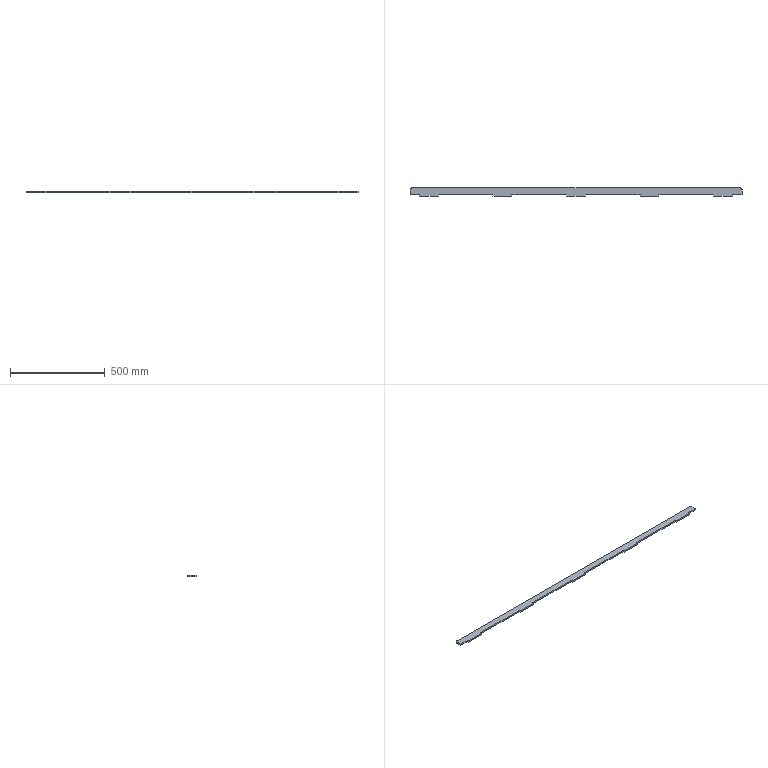Part | SolidWorks | features FlatPattern 1, SMBaseFlange 1, SheetMetal 1 | 1 solid | 28 faces | box 1750 x 42.5 x 8 mm | volume 519657 mm3 | plane 26 | cylinder 2 | commonest cylinder face diameters 20 x2
STEP:
#1=CARTESIAN_POINT('',(-889.737,-979.651,0.));
#2=VERTEX_POINT('',#1);
#3=CARTESIAN_POINT('',(-889.737,-1004.651,0.));
#4=VERTEX_POINT('',#3);
#5=CARTESIAN_POINT('',(-889.737,-1004.651,0.));
#6=DIRECTION('',(0.,-1.,0.));
#7=VECTOR('',#6,1000.);
#8=LINE('',#5,#7);
#9=EDGE_CURVE('',#2,#4,#8,.T.);
#10=ORIENTED_EDGE('',*,*,#9,.F.);
#11=CARTESIAN_POINT('',(-889.737,-979.651,-8.));
#12=VERTEX_POINT('',#11);
#13=CARTESIAN_POINT('',(-889.737,-979.651,-8.));
#14=DIRECTION('',(0.,0.,1.));
#15=VECTOR('',#14,1000.);
#16=LINE('',#13,#15);
#17=EDGE_CURVE('',#12,#2,#16,.T.);
#18=ORIENTED_EDGE('',*,*,#17,.F.);
#19=CARTESIAN_POINT('',(-889.737,-1004.651,-8.));
#20=VERTEX_POINT('',#19);
#21=CARTESIAN_POINT('',(-889.737,-1004.651,-8.));
#22=DIRECTION('',(0.,-1.,0.));
#23=VECTOR('',#22,1000.);
#24=LINE('',#21,#23);
#25=EDGE_CURVE('',#12,#20,#24,.T.);
#26=ORIENTED_EDGE('',*,*,#25,.T.);
#27=CARTESIAN_POINT('',(-889.737,-1004.651,-8.));
#28=DIRECTION('',(0.,0.,1.));
#29=VECTOR('',#28,1000.);
#30=LINE('',#27,#29);
#31=EDGE_CURVE('',#20,#4,#30,.T.);
#32=ORIENTED_EDGE('',*,*,#31,.T.);
#33=EDGE_LOOP('',(#10,#18,#26,#32));
#34=FACE_OUTER_BOUND('',#33,.T.);
#35=CARTESIAN_POINT('',(-889.737,-1004.651,-8.));
#36=DIRECTION('',(-1.,0.,0.));
#37=DIRECTION('',(0.,0.,1.));
#38=AXIS2_PLACEMENT_3D('',#35,#36,#37);
#39=PLANE('',#38);
#40=ADVANCED_FACE('',(#34),#39,.T.);
#41=CARTESIAN_POINT('',(-879.737,-969.651,0.));
#42=VERTEX_POINT('',#41);
#43=CARTESIAN_POINT('',(-879.737,-979.651,0.));
#44=DIRECTION('',(0.,0.,1.));
#45=DIRECTION('',(-1.,0.,0.));
#46=AXIS2_PLACEMENT_3D('',#43,#44,#45);
#47=CIRCLE('',#46,10.);
#48=EDGE_CURVE('',#42,#2,#47,.T.);
#49=ORIENTED_EDGE('',*,*,#48,.F.);
#50=CARTESIAN_POINT('',(-879.737,-969.651,-8.));
#51=VERTEX_POINT('',#50);
#52=CARTESIAN_POINT('',(-879.737,-969.651,-8.));
#53=DIRECTION('',(0.,0.,1.));
#54=VECTOR('',#53,1000.);
#55=LINE('',#52,#54);
#56=EDGE_CURVE('',#51,#42,#55,.T.);
#57=ORIENTED_EDGE('',*,*,#56,.F.);
#58=CARTESIAN_POINT('',(-879.737,-979.651,-8.));
#59=DIRECTION('',(0.,0.,1.));
#60=DIRECTION('',(-1.,0.,0.));
#61=AXIS2_PLACEMENT_3D('',#58,#59,#60);
#62=CIRCLE('',#61,10.);
#63=EDGE_CURVE('',#51,#12,#62,.T.);
#64=ORIENTED_EDGE('',*,*,#63,.T.);
#65=ORIENTED_EDGE('',*,*,#17,.T.);
#66=EDGE_LOOP('',(#49,#57,#64,#65));
#67=FACE_OUTER_BOUND('',#66,.T.);
#68=CARTESIAN_POINT('',(-879.737,-979.651,-8.));
#69=DIRECTION('',(0.,0.,1.));
#70=DIRECTION('',(1.,0.,0.));
#71=AXIS2_PLACEMENT_3D('',#68,#69,#70);
#72=CYLINDRICAL_SURFACE('',#71,10.);
#73=ADVANCED_FACE('',(#67),#72,.T.);
#74=CARTESIAN_POINT('',(850.263,-969.651,0.));
#75=VERTEX_POINT('',#74);
#76=CARTESIAN_POINT('',(-879.737,-969.651,0.));
#77=DIRECTION('',(-1.,0.,0.));
#78=VECTOR('',#77,1000.);
#79=LINE('',#76,#78);
#80=EDGE_CURVE('',#75,#42,#79,.T.);
#81=ORIENTED_EDGE('',*,*,#80,.F.);
#82=CARTESIAN_POINT('',(850.263,-969.651,-8.));
#83=VERTEX_POINT('',#82);
#84=CARTESIAN_POINT('',(850.263,-969.651,-8.));
#85=DIRECTION('',(0.,0.,1.));
#86=VECTOR('',#85,1000.);
#87=LINE('',#84,#86);
#88=EDGE_CURVE('',#83,#75,#87,.T.);
#89=ORIENTED_EDGE('',*,*,#88,.F.);
#90=CARTESIAN_POINT('',(-879.737,-969.651,-8.));
#91=DIRECTION('',(-1.,0.,0.));
#92=VECTOR('',#91,1000.);
#93=LINE('',#90,#92);
#94=EDGE_CURVE('',#83,#51,#93,.T.);
#95=ORIENTED_EDGE('',*,*,#94,.T.);
#96=ORIENTED_EDGE('',*,*,#56,.T.);
#97=EDGE_LOOP('',(#81,#89,#95,#96));
#98=FACE_OUTER_BOUND('',#97,.T.);
#99=CARTESIAN_POINT('',(-879.737,-969.651,-8.));
#100=DIRECTION('',(0.,1.,0.));
#101=DIRECTION('',(0.,0.,1.));
#102=AXIS2_PLACEMENT_3D('',#99,#100,#101);
#103=PLANE('',#102);
#104=ADVANCED_FACE('',(#98),#103,.T.);
#105=CARTESIAN_POINT('',(860.263,-979.651,0.));
#106=VERTEX_POINT('',#105);
#107=CARTESIAN_POINT('',(850.263,-979.651,0.));
#108=DIRECTION('',(0.,0.,1.));
#109=DIRECTION('',(-1.,0.,0.));
#110=AXIS2_PLACEMENT_3D('',#107,#108,#109);
#111=CIRCLE('',#110,10.);
#112=EDGE_CURVE('',#106,#75,#111,.T.);
#113=ORIENTED_EDGE('',*,*,#112,.F.);
#114=CARTESIAN_POINT('',(860.263,-979.651,-8.));
#115=VERTEX_POINT('',#114);
#116=CARTESIAN_POINT('',(860.263,-979.651,-8.));
#117=DIRECTION('',(0.,0.,1.));
#118=VECTOR('',#117,1000.);
#119=LINE('',#116,#118);
#120=EDGE_CURVE('',#115,#106,#119,.T.);
#121=ORIENTED_EDGE('',*,*,#120,.F.);
#122=CARTESIAN_POINT('',(850.263,-979.651,-8.));
#123=DIRECTION('',(0.,0.,1.));
#124=DIRECTION('',(-1.,0.,0.));
#125=AXIS2_PLACEMENT_3D('',#122,#123,#124);
#126=CIRCLE('',#125,10.);
#127=EDGE_CURVE('',#115,#83,#126,.T.);
#128=ORIENTED_EDGE('',*,*,#127,.T.);
#129=ORIENTED_EDGE('',*,*,#88,.T.);
#130=EDGE_LOOP('',(#113,#121,#128,#129));
#131=FACE_OUTER_BOUND('',#130,.T.);
#132=CARTESIAN_POINT('',(850.263,-979.651,-8.));
#133=DIRECTION('',(0.,0.,1.));
#134=DIRECTION('',(1.,0.,0.));
#135=AXIS2_PLACEMENT_3D('',#132,#133,#134);
#136=CYLINDRICAL_SURFACE('',#135,10.);
#137=ADVANCED_FACE('',(#131),#136,.T.);
#138=CARTESIAN_POINT('',(860.263,-1004.651,0.));
#139=VERTEX_POINT('',#138);
#140=CARTESIAN_POINT('',(860.263,-1004.651,0.));
#141=DIRECTION('',(0.,1.,0.));
#142=VECTOR('',#141,1000.);
#143=LINE('',#140,#142);
#144=EDGE_CURVE('',#139,#106,#143,.T.);
#145=ORIENTED_EDGE('',*,*,#144,.F.);
#146=CARTESIAN_POINT('',(860.263,-1004.651,-8.));
#147=VERTEX_POINT('',#146);
#148=CARTESIAN_POINT('',(860.263,-1004.651,-8.));
#149=DIRECTION('',(0.,0.,1.));
#150=VECTOR('',#149,1000.);
#151=LINE('',#148,#150);
#152=EDGE_CURVE('',#147,#139,#151,.T.);
#153=ORIENTED_EDGE('',*,*,#152,.F.);
#154=CARTESIAN_POINT('',(860.263,-1004.651,-8.));
#155=DIRECTION('',(0.,1.,0.));
#156=VECTOR('',#155,1000.);
#157=LINE('',#154,#156);
#158=EDGE_CURVE('',#147,#115,#157,.T.);
#159=ORIENTED_EDGE('',*,*,#158,.T.);
#160=ORIENTED_EDGE('',*,*,#120,.T.);
#161=EDGE_LOOP('',(#145,#153,#159,#160));
#162=FACE_OUTER_BOUND('',#161,.T.);
#163=CARTESIAN_POINT('',(860.263,-1004.651,-8.));
#164=DIRECTION('',(1.,0.,0.));
#165=DIRECTION('',(0.,0.,-1.));
#166=AXIS2_PLACEMENT_3D('',#163,#164,#165);
#167=PLANE('',#166);
#168=ADVANCED_FACE('',(#162),#167,.T.);
#169=CARTESIAN_POINT('',(810.263,-1004.651,0.));
#170=VERTEX_POINT('',#169);
#171=CARTESIAN_POINT('',(810.263,-1004.651,0.));
#172=DIRECTION('',(1.,0.,0.));
#173=VECTOR('',#172,1000.);
#174=LINE('',#171,#173);
#175=EDGE_CURVE('',#170,#139,#174,.T.);
#176=ORIENTED_EDGE('',*,*,#175,.F.);
#177=CARTESIAN_POINT('',(810.263,-1004.651,-8.));
#178=VERTEX_POINT('',#177);
#179=CARTESIAN_POINT('',(810.263,-1004.651,-8.));
#180=DIRECTION('',(0.,0.,1.));
#181=VECTOR('',#180,1000.);
#182=LINE('',#179,#181);
#183=EDGE_CURVE('',#178,#170,#182,.T.);
#184=ORIENTED_EDGE('',*,*,#183,.F.);
#185=CARTESIAN_POINT('',(810.263,-1004.651,-8.));
#186=DIRECTION('',(1.,0.,0.));
#187=VECTOR('',#186,1000.);
#188=LINE('',#185,#187);
#189=EDGE_CURVE('',#178,#147,#188,.T.);
#190=ORIENTED_EDGE('',*,*,#189,.T.);
#191=ORIENTED_EDGE('',*,*,#152,.T.);
#192=EDGE_LOOP('',(#176,#184,#190,#191));
#193=FACE_OUTER_BOUND('',#192,.T.);
#194=CARTESIAN_POINT('',(810.263,-1004.651,-8.));
#195=DIRECTION('',(0.,-1.,0.));
#196=DIRECTION('',(0.,0.,-1.));
#197=AXIS2_PLACEMENT_3D('',#194,#195,#196);
#198=PLANE('',#197);
#199=ADVANCED_FACE('',(#193),#198,.T.);
#200=CARTESIAN_POINT('',(810.263,-1012.151,0.));
#201=VERTEX_POINT('',#200);
#202=CARTESIAN_POINT('',(810.263,-1004.651,0.));
#203=DIRECTION('',(0.,1.,0.));
#204=VECTOR('',#203,1000.);
#205=LINE('',#202,#204);
#206=EDGE_CURVE('',#201,#170,#205,.T.);
#207=ORIENTED_EDGE('',*,*,#206,.F.);
#208=CARTESIAN_POINT('',(810.263,-1012.151,-8.));
#209=VERTEX_POINT('',#208);
#210=CARTESIAN_POINT('',(810.263,-1012.151,-8.));
#211=DIRECTION('',(0.,0.,1.));
#212=VECTOR('',#211,1000.);
#213=LINE('',#210,#212);
#214=EDGE_CURVE('',#209,#201,#213,.T.);
#215=ORIENTED_EDGE('',*,*,#214,.F.);
#216=CARTESIAN_POINT('',(810.263,-1004.651,-8.));
#217=DIRECTION('',(0.,1.,0.));
#218=VECTOR('',#217,1000.);
#219=LINE('',#216,#218);
#220=EDGE_CURVE('',#209,#178,#219,.T.);
#221=ORIENTED_EDGE('',*,*,#220,.T.);
#222=ORIENTED_EDGE('',*,*,#183,.T.);
#223=EDGE_LOOP('',(#207,#215,#221,#222));
#224=FACE_OUTER_BOUND('',#223,.T.);
#225=CARTESIAN_POINT('',(810.263,-1004.651,-8.));
#226=DIRECTION('',(1.,0.,0.));
#227=DIRECTION('',(0.,0.,-1.));
#228=AXIS2_PLACEMENT_3D('',#225,#226,#227);
#229=PLANE('',#228);
#230=ADVANCED_FACE('',(#224),#229,.T.);
#231=CARTESIAN_POINT('',(710.263,-1012.151,0.));
#232=VERTEX_POINT('',#231);
#233=CARTESIAN_POINT('',(810.263,-1012.151,0.));
#234=DIRECTION('',(1.,0.,0.));
#235=VECTOR('',#234,1000.);
#236=LINE('',#233,#235);
#237=EDGE_CURVE('',#232,#201,#236,.T.);
#238=ORIENTED_EDGE('',*,*,#237,.F.);
#239=CARTESIAN_POINT('',(710.263,-1012.151,-8.));
#240=VERTEX_POINT('',#239);
#241=CARTESIAN_POINT('',(710.263,-1012.151,-8.));
#242=DIRECTION('',(0.,0.,1.));
#243=VECTOR('',#242,1000.);
#244=LINE('',#241,#243);
#245=EDGE_CURVE('',#240,#232,#244,.T.);
#246=ORIENTED_EDGE('',*,*,#245,.F.);
#247=CARTESIAN_POINT('',(810.263,-1012.151,-8.));
#248=DIRECTION('',(1.,0.,0.));
#249=VECTOR('',#248,1000.);
#250=LINE('',#247,#249);
#251=EDGE_CURVE('',#240,#209,#250,.T.);
#252=ORIENTED_EDGE('',*,*,#251,.T.);
#253=ORIENTED_EDGE('',*,*,#214,.T.);
#254=EDGE_LOOP('',(#238,#246,#252,#253));
#255=FACE_OUTER_BOUND('',#254,.T.);
#256=CARTESIAN_POINT('',(810.263,-1012.151,-8.));
#257=DIRECTION('',(0.,-1.,0.));
#258=DIRECTION('',(0.,0.,-1.));
#259=AXIS2_PLACEMENT_3D('',#256,#257,#258);
#260=PLANE('',#259);
#261=ADVANCED_FACE('',(#255),#260,.T.);
#262=CARTESIAN_POINT('',(710.263,-1004.651,0.));
#263=VERTEX_POINT('',#262);
#264=CARTESIAN_POINT('',(710.263,-1012.151,0.));
#265=DIRECTION('',(0.,-1.,0.));
#266=VECTOR('',#265,1000.);
#267=LINE('',#264,#266);
#268=EDGE_CURVE('',#263,#232,#267,.T.);
#269=ORIENTED_EDGE('',*,*,#268,.F.);
#270=CARTESIAN_POINT('',(710.263,-1004.651,-8.));
#271=VERTEX_POINT('',#270);
#272=CARTESIAN_POINT('',(710.263,-1004.651,-8.));
#273=DIRECTION('',(0.,0.,1.));
#274=VECTOR('',#273,1000.);
#275=LINE('',#272,#274);
#276=EDGE_CURVE('',#271,#263,#275,.T.);
#277=ORIENTED_EDGE('',*,*,#276,.F.);
#278=CARTESIAN_POINT('',(710.263,-1012.151,-8.));
#279=DIRECTION('',(0.,-1.,0.));
#280=VECTOR('',#279,1000.);
#281=LINE('',#278,#280);
#282=EDGE_CURVE('',#271,#240,#281,.T.);
#283=ORIENTED_EDGE('',*,*,#282,.T.);
#284=ORIENTED_EDGE('',*,*,#245,.T.);
#285=EDGE_LOOP('',(#269,#277,#283,#284));
#286=FACE_OUTER_BOUND('',#285,.T.);
#287=CARTESIAN_POINT('',(710.263,-1012.151,-8.));
#288=DIRECTION('',(-1.,0.,0.));
#289=DIRECTION('',(0.,0.,1.));
#290=AXIS2_PLACEMENT_3D('',#287,#288,#289);
#291=PLANE('',#290);
#292=ADVANCED_FACE('',(#286),#291,.T.);
#293=CARTESIAN_POINT('',(422.763,-1004.651,0.));
#294=VERTEX_POINT('',#293);
#295=CARTESIAN_POINT('',(422.763,-1004.651,0.));
#296=DIRECTION('',(1.,0.,0.));
#297=VECTOR('',#296,1000.);
#298=LINE('',#295,#297);
#299=EDGE_CURVE('',#294,#263,#298,.T.);
#300=ORIENTED_EDGE('',*,*,#299,.F.);
#301=CARTESIAN_POINT('',(422.763,-1004.651,-8.));
#302=VERTEX_POINT('',#301);
#303=CARTESIAN_POINT('',(422.763,-1004.651,-8.));
#304=DIRECTION('',(0.,0.,1.));
#305=VECTOR('',#304,1000.);
#306=LINE('',#303,#305);
#307=EDGE_CURVE('',#302,#294,#306,.T.);
#308=ORIENTED_EDGE('',*,*,#307,.F.);
#309=CARTESIAN_POINT('',(422.763,-1004.651,-8.));
#310=DIRECTION('',(1.,0.,0.));
#311=VECTOR('',#310,1000.);
#312=LINE('',#309,#311);
#313=EDGE_CURVE('',#302,#271,#312,.T.);
#314=ORIENTED_EDGE('',*,*,#313,.T.);
#315=ORIENTED_EDGE('',*,*,#276,.T.);
#316=EDGE_LOOP('',(#300,#308,#314,#315));
#317=FACE_OUTER_BOUND('',#316,.T.);
#318=CARTESIAN_POINT('',(422.763,-1004.651,-8.));
#319=DIRECTION('',(0.,-1.,0.));
#320=DIRECTION('',(0.,0.,-1.));
#321=AXIS2_PLACEMENT_3D('',#318,#319,#320);
#322=PLANE('',#321);
#323=ADVANCED_FACE('',(#317),#322,.T.);
#324=CARTESIAN_POINT('',(422.763,-1012.151,0.));
#325=VERTEX_POINT('',#324);
#326=CARTESIAN_POINT('',(422.763,-1012.151,0.));
#327=DIRECTION('',(0.,1.,0.));
#328=VECTOR('',#327,1000.);
#329=LINE('',#326,#328);
#330=EDGE_CURVE('',#325,#294,#329,.T.);
#331=ORIENTED_EDGE('',*,*,#330,.F.);
#332=CARTESIAN_POINT('',(422.763,-1012.151,-8.));
#333=VERTEX_POINT('',#332);
#334=CARTESIAN_POINT('',(422.763,-1012.151,-8.));
#335=DIRECTION('',(0.,0.,1.));
#336=VECTOR('',#335,1000.);
#337=LINE('',#334,#336);
#338=EDGE_CURVE('',#333,#325,#337,.T.);
#339=ORIENTED_EDGE('',*,*,#338,.F.);
#340=CARTESIAN_POINT('',(422.763,-1012.151,-8.));
#341=DIRECTION('',(0.,1.,0.));
#342=VECTOR('',#341,1000.);
#343=LINE('',#340,#342);
#344=EDGE_CURVE('',#333,#302,#343,.T.);
#345=ORIENTED_EDGE('',*,*,#344,.T.);
#346=ORIENTED_EDGE('',*,*,#307,.T.);
#347=EDGE_LOOP('',(#331,#339,#345,#346));
#348=FACE_OUTER_BOUND('',#347,.T.);
#349=CARTESIAN_POINT('',(422.763,-1012.151,-8.));
#350=DIRECTION('',(1.,0.,0.));
#351=DIRECTION('',(0.,0.,-1.));
#352=AXIS2_PLACEMENT_3D('',#349,#350,#351);
#353=PLANE('',#352);
#354=ADVANCED_FACE('',(#348),#353,.T.);
#355=CARTESIAN_POINT('',(322.763,-1012.151,0.));
#356=VERTEX_POINT('',#355);
#357=CARTESIAN_POINT('',(322.763,-1012.151,0.));
#358=DIRECTION('',(1.,0.,0.));
#359=VECTOR('',#358,1000.);
#360=LINE('',#357,#359);
#361=EDGE_CURVE('',#356,#325,#360,.T.);
#362=ORIENTED_EDGE('',*,*,#361,.F.);
#363=CARTESIAN_POINT('',(322.763,-1012.151,-8.));
#364=VERTEX_POINT('',#363);
#365=CARTESIAN_POINT('',(322.763,-1012.151,-8.));
#366=DIRECTION('',(0.,0.,1.));
#367=VECTOR('',#366,1000.);
#368=LINE('',#365,#367);
#369=EDGE_CURVE('',#364,#356,#368,.T.);
#370=ORIENTED_EDGE('',*,*,#369,.F.);
#371=CARTESIAN_POINT('',(322.763,-1012.151,-8.));
#372=DIRECTION('',(1.,0.,0.));
#373=VECTOR('',#372,1000.);
#374=LINE('',#371,#373);
#375=EDGE_CURVE('',#364,#333,#374,.T.);
#376=ORIENTED_EDGE('',*,*,#375,.T.);
#377=ORIENTED_EDGE('',*,*,#338,.T.);
#378=EDGE_LOOP('',(#362,#370,#376,#377));
#379=FACE_OUTER_BOUND('',#378,.T.);
#380=CARTESIAN_POINT('',(322.763,-1012.151,-8.));
#381=DIRECTION('',(0.,-1.,0.));
#382=DIRECTION('',(0.,0.,-1.));
#383=AXIS2_PLACEMENT_3D('',#380,#381,#382);
#384=PLANE('',#383);
#385=ADVANCED_FACE('',(#379),#384,.T.);
#386=CARTESIAN_POINT('',(322.763,-1004.651,0.));
#387=VERTEX_POINT('',#386);
#388=CARTESIAN_POINT('',(322.763,-1004.651,0.));
#389=DIRECTION('',(0.,-1.,0.));
#390=VECTOR('',#389,1000.);
#391=LINE('',#388,#390);
#392=EDGE_CURVE('',#387,#356,#391,.T.);
#393=ORIENTED_EDGE('',*,*,#392,.F.);
#394=CARTESIAN_POINT('',(322.763,-1004.651,-8.));
#395=VERTEX_POINT('',#394);
#396=CARTESIAN_POINT('',(322.763,-1004.651,-8.));
#397=DIRECTION('',(0.,0.,1.));
#398=VECTOR('',#397,1000.);
#399=LINE('',#396,#398);
#400=EDGE_CURVE('',#395,#387,#399,.T.);
#401=ORIENTED_EDGE('',*,*,#400,.F.);
#402=CARTESIAN_POINT('',(322.763,-1004.651,-8.));
#403=DIRECTION('',(0.,-1.,0.));
#404=VECTOR('',#403,1000.);
#405=LINE('',#402,#404);
#406=EDGE_CURVE('',#395,#364,#405,.T.);
#407=ORIENTED_EDGE('',*,*,#406,.T.);
#408=ORIENTED_EDGE('',*,*,#369,.T.);
#409=EDGE_LOOP('',(#393,#401,#407,#408));
#410=FACE_OUTER_BOUND('',#409,.T.);
#411=CARTESIAN_POINT('',(322.763,-1004.651,-8.));
#412=DIRECTION('',(-1.,0.,0.));
#413=DIRECTION('',(0.,0.,1.));
#414=AXIS2_PLACEMENT_3D('',#411,#412,#413);
#415=PLANE('',#414);
#416=ADVANCED_FACE('',(#410),#415,.T.);
#417=CARTESIAN_POINT('',(35.263,-1004.651,0.));
#418=VERTEX_POINT('',#417);
#419=CARTESIAN_POINT('',(35.263,-1004.651,0.));
#420=DIRECTION('',(1.,0.,0.));
#421=VECTOR('',#420,1000.);
#422=LINE('',#419,#421);
#423=EDGE_CURVE('',#418,#387,#422,.T.);
#424=ORIENTED_EDGE('',*,*,#423,.F.);
#425=CARTESIAN_POINT('',(35.263,-1004.651,-8.));
#426=VERTEX_POINT('',#425);
#427=CARTESIAN_POINT('',(35.263,-1004.651,-8.));
#428=DIRECTION('',(0.,0.,1.));
#429=VECTOR('',#428,1000.);
#430=LINE('',#427,#429);
#431=EDGE_CURVE('',#426,#418,#430,.T.);
#432=ORIENTED_EDGE('',*,*,#431,.F.);
#433=CARTESIAN_POINT('',(35.263,-1004.651,-8.));
#434=DIRECTION('',(1.,0.,0.));
#435=VECTOR('',#434,1000.);
#436=LINE('',#433,#435);
#437=EDGE_CURVE('',#426,#395,#436,.T.);
#438=ORIENTED_EDGE('',*,*,#437,.T.);
#439=ORIENTED_EDGE('',*,*,#400,.T.);
#440=EDGE_LOOP('',(#424,#432,#438,#439));
#441=FACE_OUTER_BOUND('',#440,.T.);
#442=CARTESIAN_POINT('',(35.263,-1004.651,-8.));
#443=DIRECTION('',(0.,-1.,0.));
#444=DIRECTION('',(0.,0.,-1.));
#445=AXIS2_PLACEMENT_3D('',#442,#443,#444);
#446=PLANE('',#445);
#447=ADVANCED_FACE('',(#441),#446,.T.);
#448=CARTESIAN_POINT('',(35.263,-1012.151,0.));
#449=VERTEX_POINT('',#448);
#450=CARTESIAN_POINT('',(35.263,-1012.151,0.));
#451=DIRECTION('',(0.,1.,0.));
#452=VECTOR('',#451,1000.);
#453=LINE('',#450,#452);
#454=EDGE_CURVE('',#449,#418,#453,.T.);
#455=ORIENTED_EDGE('',*,*,#454,.F.);
#456=CARTESIAN_POINT('',(35.263,-1012.151,-8.));
#457=VERTEX_POINT('',#456);
#458=CARTESIAN_POINT('',(35.263,-1012.151,-8.));
#459=DIRECTION('',(0.,0.,1.));
#460=VECTOR('',#459,1000.);
#461=LINE('',#458,#460);
#462=EDGE_CURVE('',#457,#449,#461,.T.);
#463=ORIENTED_EDGE('',*,*,#462,.F.);
#464=CARTESIAN_POINT('',(35.263,-1012.151,-8.));
#465=DIRECTION('',(0.,1.,0.));
#466=VECTOR('',#465,1000.);
#467=LINE('',#464,#466);
#468=EDGE_CURVE('',#457,#426,#467,.T.);
#469=ORIENTED_EDGE('',*,*,#468,.T.);
#470=ORIENTED_EDGE('',*,*,#431,.T.);
#471=EDGE_LOOP('',(#455,#463,#469,#470));
#472=FACE_OUTER_BOUND('',#471,.T.);
#473=CARTESIAN_POINT('',(35.263,-1012.151,-8.));
#474=DIRECTION('',(1.,0.,0.));
#475=DIRECTION('',(0.,0.,-1.));
#476=AXIS2_PLACEMENT_3D('',#473,#474,#475);
#477=PLANE('',#476);
#478=ADVANCED_FACE('',(#472),#477,.T.);
#479=CARTESIAN_POINT('',(-64.737,-1012.151,0.));
#480=VERTEX_POINT('',#479);
#481=CARTESIAN_POINT('',(-64.737,-1012.151,0.));
#482=DIRECTION('',(1.,0.,0.));
#483=VECTOR('',#482,1000.);
#484=LINE('',#481,#483);
#485=EDGE_CURVE('',#480,#449,#484,.T.);
#486=ORIENTED_EDGE('',*,*,#485,.F.);
#487=CARTESIAN_POINT('',(-64.737,-1012.151,-8.));
#488=VERTEX_POINT('',#487);
#489=CARTESIAN_POINT('',(-64.737,-1012.151,-8.));
#490=DIRECTION('',(0.,0.,1.));
#491=VECTOR('',#490,1000.);
#492=LINE('',#489,#491);
#493=EDGE_CURVE('',#488,#480,#492,.T.);
#494=ORIENTED_EDGE('',*,*,#493,.F.);
#495=CARTESIAN_POINT('',(-64.737,-1012.151,-8.));
#496=DIRECTION('',(1.,0.,0.));
#497=VECTOR('',#496,1000.);
#498=LINE('',#495,#497);
#499=EDGE_CURVE('',#488,#457,#498,.T.);
#500=ORIENTED_EDGE('',*,*,#499,.T.);
#501=ORIENTED_EDGE('',*,*,#462,.T.);
#502=EDGE_LOOP('',(#486,#494,#500,#501));
#503=FACE_OUTER_BOUND('',#502,.T.);
#504=CARTESIAN_POINT('',(-64.737,-1012.151,-8.));
#505=DIRECTION('',(0.,-1.,0.));
#506=DIRECTION('',(0.,0.,-1.));
#507=AXIS2_PLACEMENT_3D('',#504,#505,#506);
#508=PLANE('',#507);
#509=ADVANCED_FACE('',(#503),#508,.T.);
#510=CARTESIAN_POINT('',(-64.737,-1004.651,0.));
#511=VERTEX_POINT('',#510);
#512=CARTESIAN_POINT('',(-64.737,-1004.651,0.));
#513=DIRECTION('',(0.,-1.,0.));
#514=VECTOR('',#513,1000.);
#515=LINE('',#512,#514);
#516=EDGE_CURVE('',#511,#480,#515,.T.);
#517=ORIENTED_EDGE('',*,*,#516,.F.);
#518=CARTESIAN_POINT('',(-64.737,-1004.651,-8.));
#519=VERTEX_POINT('',#518);
#520=CARTESIAN_POINT('',(-64.737,-1004.651,-8.));
#521=DIRECTION('',(0.,0.,1.));
#522=VECTOR('',#521,1000.);
#523=LINE('',#520,#522);
#524=EDGE_CURVE('',#519,#511,#523,.T.);
#525=ORIENTED_EDGE('',*,*,#524,.F.);
#526=CARTESIAN_POINT('',(-64.737,-1004.651,-8.));
#527=DIRECTION('',(0.,-1.,0.));
#528=VECTOR('',#527,1000.);
#529=LINE('',#526,#528);
#530=EDGE_CURVE('',#519,#488,#529,.T.);
#531=ORIENTED_EDGE('',*,*,#530,.T.);
#532=ORIENTED_EDGE('',*,*,#493,.T.);
#533=EDGE_LOOP('',(#517,#525,#531,#532));
#534=FACE_OUTER_BOUND('',#533,.T.);
#535=CARTESIAN_POINT('',(-64.737,-1004.651,-8.));
#536=DIRECTION('',(-1.,0.,0.));
#537=DIRECTION('',(0.,-1.,0.));
#538=AXIS2_PLACEMENT_3D('',#535,#536,#537);
#539=PLANE('',#538);
#540=ADVANCED_FACE('',(#534),#539,.T.);
#541=CARTESIAN_POINT('',(-352.237,-1004.651,0.));
#542=VERTEX_POINT('',#541);
#543=CARTESIAN_POINT('',(-352.237,-1004.651,0.));
#544=DIRECTION('',(1.,0.,0.));
#545=VECTOR('',#544,1000.);
#546=LINE('',#543,#545);
#547=EDGE_CURVE('',#542,#511,#546,.T.);
#548=ORIENTED_EDGE('',*,*,#547,.F.);
#549=CARTESIAN_POINT('',(-352.237,-1004.651,-8.));
#550=VERTEX_POINT('',#549);
#551=CARTESIAN_POINT('',(-352.237,-1004.651,-8.));
#552=DIRECTION('',(0.,0.,1.));
#553=VECTOR('',#552,1000.);
#554=LINE('',#551,#553);
#555=EDGE_CURVE('',#550,#542,#554,.T.);
#556=ORIENTED_EDGE('',*,*,#555,.F.);
#557=CARTESIAN_POINT('',(-352.237,-1004.651,-8.));
#558=DIRECTION('',(1.,0.,0.));
#559=VECTOR('',#558,1000.);
#560=LINE('',#557,#559);
#561=EDGE_CURVE('',#550,#519,#560,.T.);
#562=ORIENTED_EDGE('',*,*,#561,.T.);
#563=ORIENTED_EDGE('',*,*,#524,.T.);
#564=EDGE_LOOP('',(#548,#556,#562,#563));
#565=FACE_OUTER_BOUND('',#564,.T.);
#566=CARTESIAN_POINT('',(-352.237,-1004.651,-8.));
#567=DIRECTION('',(0.,-1.,0.));
#568=DIRECTION('',(0.,0.,-1.));
#569=AXIS2_PLACEMENT_3D('',#566,#567,#568);
#570=PLANE('',#569);
#571=ADVANCED_FACE('',(#565),#570,.T.);
#572=CARTESIAN_POINT('',(-352.237,-1012.151,0.));
#573=VERTEX_POINT('',#572);
#574=CARTESIAN_POINT('',(-352.237,-1012.151,0.));
#575=DIRECTION('',(0.,1.,0.));
#576=VECTOR('',#575,1000.);
#577=LINE('',#574,#576);
#578=EDGE_CURVE('',#573,#542,#577,.T.);
#579=ORIENTED_EDGE('',*,*,#578,.F.);
#580=CARTESIAN_POINT('',(-352.237,-1012.151,-8.));
#581=VERTEX_POINT('',#580);
#582=CARTESIAN_POINT('',(-352.237,-1012.151,-8.));
#583=DIRECTION('',(0.,0.,1.));
#584=VECTOR('',#583,1000.);
#585=LINE('',#582,#584);
#586=EDGE_CURVE('',#581,#573,#585,.T.);
#587=ORIENTED_EDGE('',*,*,#586,.F.);
#588=CARTESIAN_POINT('',(-352.237,-1012.151,-8.));
#589=DIRECTION('',(0.,1.,0.));
#590=VECTOR('',#589,1000.);
#591=LINE('',#588,#590);
#592=EDGE_CURVE('',#581,#550,#591,.T.);
#593=ORIENTED_EDGE('',*,*,#592,.T.);
#594=ORIENTED_EDGE('',*,*,#555,.T.);
#595=EDGE_LOOP('',(#579,#587,#593,#594));
#596=FACE_OUTER_BOUND('',#595,.T.);
#597=CARTESIAN_POINT('',(-352.237,-1012.151,-8.));
#598=DIRECTION('',(1.,0.,0.));
#599=DIRECTION('',(0.,0.,-1.));
#600=AXIS2_PLACEMENT_3D('',#597,#598,#599);
#601=PLANE('',#600);
#602=ADVANCED_FACE('',(#596),#601,.T.);
#603=CARTESIAN_POINT('',(-452.237,-1012.151,0.));
#604=VERTEX_POINT('',#603);
#605=CARTESIAN_POINT('',(-452.237,-1012.151,0.));
#606=DIRECTION('',(1.,0.,0.));
#607=VECTOR('',#606,1000.);
#608=LINE('',#605,#607);
#609=EDGE_CURVE('',#604,#573,#608,.T.);
#610=ORIENTED_EDGE('',*,*,#609,.F.);
#611=CARTESIAN_POINT('',(-452.237,-1012.151,-8.));
#612=VERTEX_POINT('',#611);
#613=CARTESIAN_POINT('',(-452.237,-1012.151,-8.));
#614=DIRECTION('',(0.,0.,1.));
#615=VECTOR('',#614,1000.);
#616=LINE('',#613,#615);
#617=EDGE_CURVE('',#612,#604,#616,.T.);
#618=ORIENTED_EDGE('',*,*,#617,.F.);
#619=CARTESIAN_POINT('',(-452.237,-1012.151,-8.));
#620=DIRECTION('',(1.,0.,0.));
#621=VECTOR('',#620,1000.);
#622=LINE('',#619,#621);
#623=EDGE_CURVE('',#612,#581,#622,.T.);
#624=ORIENTED_EDGE('',*,*,#623,.T.);
#625=ORIENTED_EDGE('',*,*,#586,.T.);
#626=EDGE_LOOP('',(#610,#618,#624,#625));
#627=FACE_OUTER_BOUND('',#626,.T.);
#628=CARTESIAN_POINT('',(-452.237,-1012.151,-8.));
#629=DIRECTION('',(0.,-1.,0.));
#630=DIRECTION('',(0.,0.,-1.));
#631=AXIS2_PLACEMENT_3D('',#628,#629,#630);
#632=PLANE('',#631);
#633=ADVANCED_FACE('',(#627),#632,.T.);
#634=CARTESIAN_POINT('',(-452.237,-1004.651,0.));
#635=VERTEX_POINT('',#634);
#636=CARTESIAN_POINT('',(-452.237,-1004.651,0.));
#637=DIRECTION('',(0.,-1.,0.));
#638=VECTOR('',#637,1000.);
#639=LINE('',#636,#638);
#640=EDGE_CURVE('',#635,#604,#639,.T.);
#641=ORIENTED_EDGE('',*,*,#640,.F.);
#642=CARTESIAN_POINT('',(-452.237,-1004.651,-8.));
#643=VERTEX_POINT('',#642);
#644=CARTESIAN_POINT('',(-452.237,-1004.651,-8.));
#645=DIRECTION('',(0.,0.,1.));
#646=VECTOR('',#645,1000.);
#647=LINE('',#644,#646);
#648=EDGE_CURVE('',#643,#635,#647,.T.);
#649=ORIENTED_EDGE('',*,*,#648,.F.);
#650=CARTESIAN_POINT('',(-452.237,-1004.651,-8.));
#651=DIRECTION('',(0.,-1.,0.));
#652=VECTOR('',#651,1000.);
#653=LINE('',#650,#652);
#654=EDGE_CURVE('',#643,#612,#653,.T.);
#655=ORIENTED_EDGE('',*,*,#654,.T.);
#656=ORIENTED_EDGE('',*,*,#617,.T.);
#657=EDGE_LOOP('',(#641,#649,#655,#656));
#658=FACE_OUTER_BOUND('',#657,.T.);
#659=CARTESIAN_POINT('',(-452.237,-1004.651,-8.));
#660=DIRECTION('',(-1.,0.,0.));
#661=DIRECTION('',(0.,0.,1.));
#662=AXIS2_PLACEMENT_3D('',#659,#660,#661);
#663=PLANE('',#662);
#664=ADVANCED_FACE('',(#658),#663,.T.);
#665=CARTESIAN_POINT('',(-739.737,-1004.651,0.));
#666=VERTEX_POINT('',#665);
#667=CARTESIAN_POINT('',(-739.737,-1004.651,0.));
#668=DIRECTION('',(1.,0.,0.));
#669=VECTOR('',#668,1000.);
#670=LINE('',#667,#669);
#671=EDGE_CURVE('',#666,#635,#670,.T.);
#672=ORIENTED_EDGE('',*,*,#671,.F.);
#673=CARTESIAN_POINT('',(-739.737,-1004.651,-8.));
#674=VERTEX_POINT('',#673);
#675=CARTESIAN_POINT('',(-739.737,-1004.651,-8.));
#676=DIRECTION('',(0.,0.,1.));
#677=VECTOR('',#676,1000.);
#678=LINE('',#675,#677);
#679=EDGE_CURVE('',#674,#666,#678,.T.);
#680=ORIENTED_EDGE('',*,*,#679,.F.);
#681=CARTESIAN_POINT('',(-739.737,-1004.651,-8.));
#682=DIRECTION('',(1.,0.,0.));
#683=VECTOR('',#682,1000.);
#684=LINE('',#681,#683);
#685=EDGE_CURVE('',#674,#643,#684,.T.);
#686=ORIENTED_EDGE('',*,*,#685,.T.);
#687=ORIENTED_EDGE('',*,*,#648,.T.);
#688=EDGE_LOOP('',(#672,#680,#686,#687));
#689=FACE_OUTER_BOUND('',#688,.T.);
#690=CARTESIAN_POINT('',(-739.737,-1004.651,-8.));
#691=DIRECTION('',(0.,-1.,0.));
#692=DIRECTION('',(0.,0.,-1.));
#693=AXIS2_PLACEMENT_3D('',#690,#691,#692);
#694=PLANE('',#693);
#695=ADVANCED_FACE('',(#689),#694,.T.);
#696=CARTESIAN_POINT('',(-739.737,-1012.151,0.));
#697=VERTEX_POINT('',#696);
#698=CARTESIAN_POINT('',(-739.737,-1012.151,0.));
#699=DIRECTION('',(0.,1.,0.));
#700=VECTOR('',#699,1000.);
#701=LINE('',#698,#700);
#702=EDGE_CURVE('',#697,#666,#701,.T.);
#703=ORIENTED_EDGE('',*,*,#702,.F.);
#704=CARTESIAN_POINT('',(-739.737,-1012.151,-8.));
#705=VERTEX_POINT('',#704);
#706=CARTESIAN_POINT('',(-739.737,-1012.151,-8.));
#707=DIRECTION('',(0.,0.,1.));
#708=VECTOR('',#707,1000.);
#709=LINE('',#706,#708);
#710=EDGE_CURVE('',#705,#697,#709,.T.);
#711=ORIENTED_EDGE('',*,*,#710,.F.);
#712=CARTESIAN_POINT('',(-739.737,-1012.151,-8.));
#713=DIRECTION('',(0.,1.,0.));
#714=VECTOR('',#713,1000.);
#715=LINE('',#712,#714);
#716=EDGE_CURVE('',#705,#674,#715,.T.);
#717=ORIENTED_EDGE('',*,*,#716,.T.);
#718=ORIENTED_EDGE('',*,*,#679,.T.);
#719=EDGE_LOOP('',(#703,#711,#717,#718));
#720=FACE_OUTER_BOUND('',#719,.T.);
#721=CARTESIAN_POINT('',(-739.737,-1012.151,-8.));
#722=DIRECTION('',(1.,0.,0.));
#723=DIRECTION('',(0.,0.,-1.));
#724=AXIS2_PLACEMENT_3D('',#721,#722,#723);
#725=PLANE('',#724);
#726=ADVANCED_FACE('',(#720),#725,.T.);
#727=CARTESIAN_POINT('',(-839.737,-1012.151,0.));
#728=VERTEX_POINT('',#727);
#729=CARTESIAN_POINT('',(-839.737,-1012.151,0.));
#730=DIRECTION('',(1.,0.,0.));
#731=VECTOR('',#730,1000.);
#732=LINE('',#729,#731);
#733=EDGE_CURVE('',#728,#697,#732,.T.);
#734=ORIENTED_EDGE('',*,*,#733,.F.);
#735=CARTESIAN_POINT('',(-839.737,-1012.151,-8.));
#736=VERTEX_POINT('',#735);
#737=CARTESIAN_POINT('',(-839.737,-1012.151,-8.));
#738=DIRECTION('',(0.,0.,1.));
#739=VECTOR('',#738,1000.);
#740=LINE('',#737,#739);
#741=EDGE_CURVE('',#736,#728,#740,.T.);
#742=ORIENTED_EDGE('',*,*,#741,.F.);
#743=CARTESIAN_POINT('',(-839.737,-1012.151,-8.));
#744=DIRECTION('',(1.,0.,0.));
#745=VECTOR('',#744,1000.);
#746=LINE('',#743,#745);
#747=EDGE_CURVE('',#736,#705,#746,.T.);
#748=ORIENTED_EDGE('',*,*,#747,.T.);
#749=ORIENTED_EDGE('',*,*,#710,.T.);
#750=EDGE_LOOP('',(#734,#742,#748,#749));
#751=FACE_OUTER_BOUND('',#750,.T.);
#752=CARTESIAN_POINT('',(-839.737,-1012.151,-8.));
#753=DIRECTION('',(0.,-1.,0.));
#754=DIRECTION('',(1.,0.,0.));
#755=AXIS2_PLACEMENT_3D('',#752,#753,#754);
#756=PLANE('',#755);
#757=ADVANCED_FACE('',(#751),#756,.T.);
#758=CARTESIAN_POINT('',(-839.737,-1004.651,0.));
#759=VERTEX_POINT('',#758);
#760=CARTESIAN_POINT('',(-839.737,-1004.651,0.));
#761=DIRECTION('',(0.,-1.,0.));
#762=VECTOR('',#761,1000.);
#763=LINE('',#760,#762);
#764=EDGE_CURVE('',#759,#728,#763,.T.);
#765=ORIENTED_EDGE('',*,*,#764,.F.);
#766=CARTESIAN_POINT('',(-839.737,-1004.651,-8.));
#767=VERTEX_POINT('',#766);
#768=CARTESIAN_POINT('',(-839.737,-1004.651,-8.));
#769=DIRECTION('',(0.,0.,1.));
#770=VECTOR('',#769,1000.);
#771=LINE('',#768,#770);
#772=EDGE_CURVE('',#767,#759,#771,.T.);
#773=ORIENTED_EDGE('',*,*,#772,.F.);
#774=CARTESIAN_POINT('',(-839.737,-1004.651,-8.));
#775=DIRECTION('',(0.,-1.,0.));
#776=VECTOR('',#775,1000.);
#777=LINE('',#774,#776);
#778=EDGE_CURVE('',#767,#736,#777,.T.);
#779=ORIENTED_EDGE('',*,*,#778,.T.);
#780=ORIENTED_EDGE('',*,*,#741,.T.);
#781=EDGE_LOOP('',(#765,#773,#779,#780));
#782=FACE_OUTER_BOUND('',#781,.T.);
#783=CARTESIAN_POINT('',(-839.737,-1004.651,-8.));
#784=DIRECTION('',(-1.,0.,0.));
#785=DIRECTION('',(0.,0.,1.));
#786=AXIS2_PLACEMENT_3D('',#783,#784,#785);
#787=PLANE('',#786);
#788=ADVANCED_FACE('',(#782),#787,.T.);
#789=CARTESIAN_POINT('',(-889.737,-1004.651,0.));
#790=DIRECTION('',(1.,0.,0.));
#791=VECTOR('',#790,1000.);
#792=LINE('',#789,#791);
#793=EDGE_CURVE('',#4,#759,#792,.T.);
#794=ORIENTED_EDGE('',*,*,#793,.F.);
#795=ORIENTED_EDGE('',*,*,#31,.F.);
#796=CARTESIAN_POINT('',(-889.737,-1004.651,-8.));
#797=DIRECTION('',(1.,0.,0.));
#798=VECTOR('',#797,1000.);
#799=LINE('',#796,#798);
#800=EDGE_CURVE('',#20,#767,#799,.T.);
#801=ORIENTED_EDGE('',*,*,#800,.T.);
#802=ORIENTED_EDGE('',*,*,#772,.T.);
#803=EDGE_LOOP('',(#794,#795,#801,#802));
#804=FACE_OUTER_BOUND('',#803,.T.);
#805=CARTESIAN_POINT('',(-889.737,-1004.651,-8.));
#806=DIRECTION('',(0.,-1.,0.));
#807=DIRECTION('',(0.,0.,-1.));
#808=AXIS2_PLACEMENT_3D('',#805,#806,#807);
#809=PLANE('',#808);
#810=ADVANCED_FACE('',(#804),#809,.T.);
#811=ORIENTED_EDGE('',*,*,#25,.F.);
#812=ORIENTED_EDGE('',*,*,#63,.F.);
#813=ORIENTED_EDGE('',*,*,#94,.F.);
#814=ORIENTED_EDGE('',*,*,#127,.F.);
#815=ORIENTED_EDGE('',*,*,#158,.F.);
#816=ORIENTED_EDGE('',*,*,#189,.F.);
#817=ORIENTED_EDGE('',*,*,#220,.F.);
#818=ORIENTED_EDGE('',*,*,#251,.F.);
#819=ORIENTED_EDGE('',*,*,#282,.F.);
#820=ORIENTED_EDGE('',*,*,#313,.F.);
#821=ORIENTED_EDGE('',*,*,#344,.F.);
#822=ORIENTED_EDGE('',*,*,#375,.F.);
#823=ORIENTED_EDGE('',*,*,#406,.F.);
#824=ORIENTED_EDGE('',*,*,#437,.F.);
#825=ORIENTED_EDGE('',*,*,#468,.F.);
#826=ORIENTED_EDGE('',*,*,#499,.F.);
#827=ORIENTED_EDGE('',*,*,#530,.F.);
#828=ORIENTED_EDGE('',*,*,#561,.F.);
#829=ORIENTED_EDGE('',*,*,#592,.F.);
#830=ORIENTED_EDGE('',*,*,#623,.F.);
#831=ORIENTED_EDGE('',*,*,#654,.F.);
#832=ORIENTED_EDGE('',*,*,#685,.F.);
#833=ORIENTED_EDGE('',*,*,#716,.F.);
#834=ORIENTED_EDGE('',*,*,#747,.F.);
#835=ORIENTED_EDGE('',*,*,#778,.F.);
#836=ORIENTED_EDGE('',*,*,#800,.F.);
#837=EDGE_LOOP('',(#811,#812,#813,#814,#815,#816,#817,#818,#819,#820,#821,#822,#823,#824,#825,#826,#827,#828,#829,#830,#831,#832,#833,#834,#835,#836));
#838=FACE_OUTER_BOUND('',#837,.T.);
#839=CARTESIAN_POINT('',(-879.737,-979.651,-8.));
#840=DIRECTION('',(0.,0.,-1.));
#841=DIRECTION('',(-1.,0.,0.));
#842=AXIS2_PLACEMENT_3D('',#839,#840,#841);
#843=PLANE('',#842);
#844=ADVANCED_FACE('',(#838),#843,.T.);
#845=ORIENTED_EDGE('',*,*,#9,.T.);
#846=ORIENTED_EDGE('',*,*,#793,.T.);
#847=ORIENTED_EDGE('',*,*,#764,.T.);
#848=ORIENTED_EDGE('',*,*,#733,.T.);
#849=ORIENTED_EDGE('',*,*,#702,.T.);
#850=ORIENTED_EDGE('',*,*,#671,.T.);
#851=ORIENTED_EDGE('',*,*,#640,.T.);
#852=ORIENTED_EDGE('',*,*,#609,.T.);
#853=ORIENTED_EDGE('',*,*,#578,.T.);
#854=ORIENTED_EDGE('',*,*,#547,.T.);
#855=ORIENTED_EDGE('',*,*,#516,.T.);
#856=ORIENTED_EDGE('',*,*,#485,.T.);
#857=ORIENTED_EDGE('',*,*,#454,.T.);
#858=ORIENTED_EDGE('',*,*,#423,.T.);
#859=ORIENTED_EDGE('',*,*,#392,.T.);
#860=ORIENTED_EDGE('',*,*,#361,.T.);
#861=ORIENTED_EDGE('',*,*,#330,.T.);
#862=ORIENTED_EDGE('',*,*,#299,.T.);
#863=ORIENTED_EDGE('',*,*,#268,.T.);
#864=ORIENTED_EDGE('',*,*,#237,.T.);
#865=ORIENTED_EDGE('',*,*,#206,.T.);
#866=ORIENTED_EDGE('',*,*,#175,.T.);
#867=ORIENTED_EDGE('',*,*,#144,.T.);
#868=ORIENTED_EDGE('',*,*,#112,.T.);
#869=ORIENTED_EDGE('',*,*,#80,.T.);
#870=ORIENTED_EDGE('',*,*,#48,.T.);
#871=EDGE_LOOP('',(#845,#846,#847,#848,#849,#850,#851,#852,#853,#854,#855,#856,#857,#858,#859,#860,#861,#862,#863,#864,#865,#866,#867,#868,#869,#870));
#872=FACE_OUTER_BOUND('',#871,.T.);
#873=CARTESIAN_POINT('',(-879.737,-979.651,0.));
#874=DIRECTION('',(0.,0.,-1.));
#875=DIRECTION('',(-1.,0.,0.));
#876=AXIS2_PLACEMENT_3D('',#873,#874,#875);
#877=PLANE('',#876);
#878=ADVANCED_FACE('',(#872),#877,.F.);
#879=CLOSED_SHELL('',(#40,#73,#104,#137,#168,#199,#230,#261,#292,#323,#354,#385,#416,#447,#478,#509,#540,#571,#602,#633,#664,#695,#726,#757,#788,#810,#844,#878));
#880=MANIFOLD_SOLID_BREP('',#879);
#881=CARTESIAN_POINT('',(0.,0.,0.));
#882=DIRECTION('',(0.,0.,1.));
#883=DIRECTION('',(1.,0.,0.));
#884=AXIS2_PLACEMENT_3D('',#881,#882,#883);
#885=(LENGTH_UNIT()NAMED_UNIT(*)SI_UNIT(.MILLI.,.METRE.));
#886=UNCERTAINTY_MEASURE_WITH_UNIT(LENGTH_MEASURE(0.00001),#885,'','');
#887=(NAMED_UNIT(*)PLANE_ANGLE_UNIT()SI_UNIT($,.RADIAN.));
#888=(NAMED_UNIT(*)SI_UNIT($,.STERADIAN.)SOLID_ANGLE_UNIT());
#889=(GEOMETRIC_REPRESENTATION_CONTEXT(3)GLOBAL_UNCERTAINTY_ASSIGNED_CONTEXT((#886))GLOBAL_UNIT_ASSIGNED_CONTEXT((#885,#887,#888))REPRESENTATION_CONTEXT('',''));
#890=ADVANCED_BREP_SHAPE_REPRESENTATION('',(#880,#884),#889);